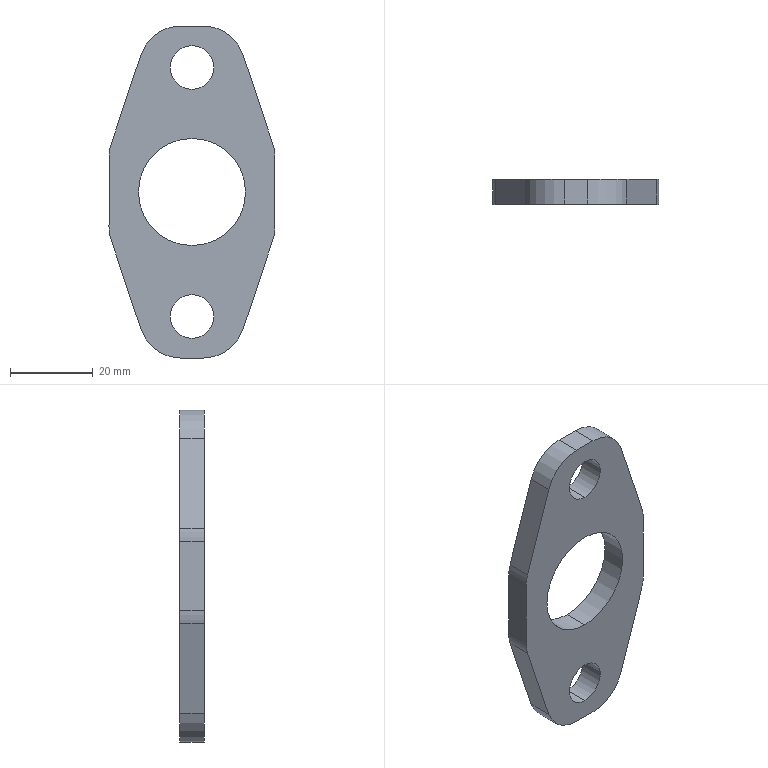Part | SolidWorks | features BaseBody 1 | 1 solid | 24 faces | box 40 x 6 x 80 mm | volume 11190 mm3 | cylinder 14 | plane 10 | commonest cylinder face diameters 20 x8 10.5 x4 25.8 x2
STEP:
#1=CARTESIAN_POINT('',(921.946,-3040.973,882.071));
#2=VERTEX_POINT('',#1);
#3=CARTESIAN_POINT('',(921.946,-3040.973,907.871));
#4=VERTEX_POINT('',#3);
#5=CARTESIAN_POINT('',(921.946,-3040.973,894.971));
#6=DIRECTION('',(0.,1.,0.));
#7=DIRECTION('',(0.,0.,-1.));
#8=AXIS2_PLACEMENT_3D('',#5,#6,#7);
#9=CIRCLE('',#8,12.9);
#10=EDGE_CURVE('',#2,#4,#9,.T.);
#11=ORIENTED_EDGE('',*,*,#10,.T.);
#12=CARTESIAN_POINT('',(921.946,-3046.973,907.871));
#13=VERTEX_POINT('',#12);
#14=CARTESIAN_POINT('',(921.946,-3040.973,907.871));
#15=DIRECTION('',(0.,-1.,0.));
#16=VECTOR('',#15,1000.);
#17=LINE('',#14,#16);
#18=EDGE_CURVE('',#4,#13,#17,.T.);
#19=ORIENTED_EDGE('',*,*,#18,.T.);
#20=CARTESIAN_POINT('',(921.946,-3046.973,882.071));
#21=VERTEX_POINT('',#20);
#22=CARTESIAN_POINT('',(921.946,-3046.973,894.971));
#23=DIRECTION('',(0.,-1.,0.));
#24=DIRECTION('',(0.,0.,-1.));
#25=AXIS2_PLACEMENT_3D('',#22,#23,#24);
#26=CIRCLE('',#25,12.9);
#27=EDGE_CURVE('',#13,#21,#26,.T.);
#28=ORIENTED_EDGE('',*,*,#27,.T.);
#29=CARTESIAN_POINT('',(921.946,-3040.973,882.071));
#30=DIRECTION('',(0.,-1.,0.));
#31=VECTOR('',#30,1000.);
#32=LINE('',#29,#31);
#33=EDGE_CURVE('',#2,#21,#32,.T.);
#34=ORIENTED_EDGE('',*,*,#33,.F.);
#35=EDGE_LOOP('',(#11,#19,#28,#34));
#36=FACE_OUTER_BOUND('',#35,.T.);
#37=CARTESIAN_POINT('',(921.946,-3040.973,894.971));
#38=DIRECTION('',(0.,-1.,0.));
#39=DIRECTION('',(0.,0.,-1.));
#40=AXIS2_PLACEMENT_3D('',#37,#38,#39);
#41=CYLINDRICAL_SURFACE('',#40,12.9);
#42=ADVANCED_FACE('',(#36),#41,.F.);
#43=CARTESIAN_POINT('',(921.946,-3040.973,859.721));
#44=VERTEX_POINT('',#43);
#45=CARTESIAN_POINT('',(921.946,-3040.973,870.221));
#46=VERTEX_POINT('',#45);
#47=CARTESIAN_POINT('',(921.946,-3040.973,864.971));
#48=DIRECTION('',(0.,1.,0.));
#49=DIRECTION('',(0.,0.,-1.));
#50=AXIS2_PLACEMENT_3D('',#47,#48,#49);
#51=CIRCLE('',#50,5.25);
#52=EDGE_CURVE('',#44,#46,#51,.T.);
#53=ORIENTED_EDGE('',*,*,#52,.T.);
#54=CARTESIAN_POINT('',(921.946,-3046.973,870.221));
#55=VERTEX_POINT('',#54);
#56=CARTESIAN_POINT('',(921.946,-3040.973,870.221));
#57=DIRECTION('',(0.,-1.,0.));
#58=VECTOR('',#57,1000.);
#59=LINE('',#56,#58);
#60=EDGE_CURVE('',#46,#55,#59,.T.);
#61=ORIENTED_EDGE('',*,*,#60,.T.);
#62=CARTESIAN_POINT('',(921.946,-3046.973,859.721));
#63=VERTEX_POINT('',#62);
#64=CARTESIAN_POINT('',(921.946,-3046.973,864.971));
#65=DIRECTION('',(0.,-1.,0.));
#66=DIRECTION('',(0.,0.,-1.));
#67=AXIS2_PLACEMENT_3D('',#64,#65,#66);
#68=CIRCLE('',#67,5.25);
#69=EDGE_CURVE('',#55,#63,#68,.T.);
#70=ORIENTED_EDGE('',*,*,#69,.T.);
#71=CARTESIAN_POINT('',(921.946,-3040.973,859.721));
#72=DIRECTION('',(0.,-1.,0.));
#73=VECTOR('',#72,1000.);
#74=LINE('',#71,#73);
#75=EDGE_CURVE('',#44,#63,#74,.T.);
#76=ORIENTED_EDGE('',*,*,#75,.F.);
#77=EDGE_LOOP('',(#53,#61,#70,#76));
#78=FACE_OUTER_BOUND('',#77,.T.);
#79=CARTESIAN_POINT('',(921.946,-3040.973,864.971));
#80=DIRECTION('',(0.,-1.,0.));
#81=DIRECTION('',(0.,0.,-1.));
#82=AXIS2_PLACEMENT_3D('',#79,#80,#81);
#83=CYLINDRICAL_SURFACE('',#82,5.25);
#84=ADVANCED_FACE('',(#78),#83,.F.);
#85=CARTESIAN_POINT('',(921.946,-3040.973,919.721));
#86=VERTEX_POINT('',#85);
#87=CARTESIAN_POINT('',(921.946,-3040.973,930.221));
#88=VERTEX_POINT('',#87);
#89=CARTESIAN_POINT('',(921.946,-3040.973,924.971));
#90=DIRECTION('',(0.,1.,0.));
#91=DIRECTION('',(0.,0.,-1.));
#92=AXIS2_PLACEMENT_3D('',#89,#90,#91);
#93=CIRCLE('',#92,5.25);
#94=EDGE_CURVE('',#86,#88,#93,.T.);
#95=ORIENTED_EDGE('',*,*,#94,.T.);
#96=CARTESIAN_POINT('',(921.946,-3046.973,930.221));
#97=VERTEX_POINT('',#96);
#98=CARTESIAN_POINT('',(921.946,-3040.973,930.221));
#99=DIRECTION('',(0.,-1.,0.));
#100=VECTOR('',#99,1000.);
#101=LINE('',#98,#100);
#102=EDGE_CURVE('',#88,#97,#101,.T.);
#103=ORIENTED_EDGE('',*,*,#102,.T.);
#104=CARTESIAN_POINT('',(921.946,-3046.973,919.721));
#105=VERTEX_POINT('',#104);
#106=CARTESIAN_POINT('',(921.946,-3046.973,924.971));
#107=DIRECTION('',(0.,-1.,0.));
#108=DIRECTION('',(0.,0.,-1.));
#109=AXIS2_PLACEMENT_3D('',#106,#107,#108);
#110=CIRCLE('',#109,5.25);
#111=EDGE_CURVE('',#97,#105,#110,.T.);
#112=ORIENTED_EDGE('',*,*,#111,.T.);
#113=CARTESIAN_POINT('',(921.946,-3040.973,919.721));
#114=DIRECTION('',(0.,-1.,0.));
#115=VECTOR('',#114,1000.);
#116=LINE('',#113,#115);
#117=EDGE_CURVE('',#86,#105,#116,.T.);
#118=ORIENTED_EDGE('',*,*,#117,.F.);
#119=EDGE_LOOP('',(#95,#103,#112,#118));
#120=FACE_OUTER_BOUND('',#119,.T.);
#121=CARTESIAN_POINT('',(921.946,-3040.973,924.971));
#122=DIRECTION('',(0.,-1.,0.));
#123=DIRECTION('',(0.,0.,-1.));
#124=AXIS2_PLACEMENT_3D('',#121,#122,#123);
#125=CYLINDRICAL_SURFACE('',#124,5.25);
#126=ADVANCED_FACE('',(#120),#125,.F.);
#127=CARTESIAN_POINT('',(941.946,-3046.973,886.594));
#128=VERTEX_POINT('',#127);
#129=CARTESIAN_POINT('',(941.432,-3046.973,883.432));
#130=VERTEX_POINT('',#129);
#131=CARTESIAN_POINT('',(931.946,-3046.973,886.594));
#132=DIRECTION('',(0.,1.,0.));
#133=DIRECTION('',(0.,0.,-1.));
#134=AXIS2_PLACEMENT_3D('',#131,#132,#133);
#135=CIRCLE('',#134,10.);
#136=EDGE_CURVE('',#128,#130,#135,.T.);
#137=ORIENTED_EDGE('',*,*,#136,.F.);
#138=CARTESIAN_POINT('',(941.946,-3046.973,903.349));
#139=VERTEX_POINT('',#138);
#140=CARTESIAN_POINT('',(941.946,-3046.973,894.971));
#141=DIRECTION('',(0.,0.,-1.));
#142=VECTOR('',#141,1000.);
#143=LINE('',#140,#142);
#144=EDGE_CURVE('',#139,#128,#143,.T.);
#145=ORIENTED_EDGE('',*,*,#144,.F.);
#146=CARTESIAN_POINT('',(941.432,-3046.973,906.511));
#147=VERTEX_POINT('',#146);
#148=CARTESIAN_POINT('',(931.946,-3046.973,903.349));
#149=DIRECTION('',(0.,1.,0.));
#150=DIRECTION('',(0.,0.,-1.));
#151=AXIS2_PLACEMENT_3D('',#148,#149,#150);
#152=CIRCLE('',#151,10.);
#153=EDGE_CURVE('',#147,#139,#152,.T.);
#154=ORIENTED_EDGE('',*,*,#153,.F.);
#155=CARTESIAN_POINT('',(934.225,-3046.973,928.134));
#156=VERTEX_POINT('',#155);
#157=CARTESIAN_POINT('',(934.225,-3046.973,928.134));
#158=DIRECTION('',(0.3162,0.,-0.9487));
#159=VECTOR('',#158,1000.);
#160=LINE('',#157,#159);
#161=EDGE_CURVE('',#156,#147,#160,.T.);
#162=ORIENTED_EDGE('',*,*,#161,.F.);
#163=CARTESIAN_POINT('',(924.738,-3046.973,934.971));
#164=VERTEX_POINT('',#163);
#165=CARTESIAN_POINT('',(924.738,-3046.973,924.971));
#166=DIRECTION('',(0.,1.,0.));
#167=DIRECTION('',(0.,0.,-1.));
#168=AXIS2_PLACEMENT_3D('',#165,#166,#167);
#169=CIRCLE('',#168,10.);
#170=EDGE_CURVE('',#164,#156,#169,.T.);
#171=ORIENTED_EDGE('',*,*,#170,.F.);
#172=CARTESIAN_POINT('',(919.153,-3046.973,934.971));
#173=VERTEX_POINT('',#172);
#174=CARTESIAN_POINT('',(921.946,-3046.973,934.971));
#175=DIRECTION('',(1.,0.,0.));
#176=VECTOR('',#175,1000.);
#177=LINE('',#174,#176);
#178=EDGE_CURVE('',#173,#164,#177,.T.);
#179=ORIENTED_EDGE('',*,*,#178,.F.);
#180=CARTESIAN_POINT('',(909.666,-3046.973,928.134));
#181=VERTEX_POINT('',#180);
#182=CARTESIAN_POINT('',(919.153,-3046.973,924.971));
#183=DIRECTION('',(0.,1.,0.));
#184=DIRECTION('',(0.,0.,-1.));
#185=AXIS2_PLACEMENT_3D('',#182,#183,#184);
#186=CIRCLE('',#185,10.);
#187=EDGE_CURVE('',#181,#173,#186,.T.);
#188=ORIENTED_EDGE('',*,*,#187,.F.);
#189=CARTESIAN_POINT('',(902.459,-3046.973,906.511));
#190=VERTEX_POINT('',#189);
#191=CARTESIAN_POINT('',(902.459,-3046.973,906.511));
#192=DIRECTION('',(0.3162,0.,0.9487));
#193=VECTOR('',#192,1000.);
#194=LINE('',#191,#193);
#195=EDGE_CURVE('',#190,#181,#194,.T.);
#196=ORIENTED_EDGE('',*,*,#195,.F.);
#197=CARTESIAN_POINT('',(901.946,-3046.973,903.349));
#198=VERTEX_POINT('',#197);
#199=CARTESIAN_POINT('',(911.946,-3046.973,903.349));
#200=DIRECTION('',(0.,1.,0.));
#201=DIRECTION('',(0.,0.,-1.));
#202=AXIS2_PLACEMENT_3D('',#199,#200,#201);
#203=CIRCLE('',#202,10.);
#204=EDGE_CURVE('',#198,#190,#203,.T.);
#205=ORIENTED_EDGE('',*,*,#204,.F.);
#206=CARTESIAN_POINT('',(901.946,-3046.973,886.594));
#207=VERTEX_POINT('',#206);
#208=CARTESIAN_POINT('',(901.946,-3046.973,894.971));
#209=DIRECTION('',(0.,0.,1.));
#210=VECTOR('',#209,1000.);
#211=LINE('',#208,#210);
#212=EDGE_CURVE('',#207,#198,#211,.T.);
#213=ORIENTED_EDGE('',*,*,#212,.F.);
#214=CARTESIAN_POINT('',(902.459,-3046.973,883.432));
#215=VERTEX_POINT('',#214);
#216=CARTESIAN_POINT('',(911.946,-3046.973,886.594));
#217=DIRECTION('',(0.,1.,0.));
#218=DIRECTION('',(0.,0.,-1.));
#219=AXIS2_PLACEMENT_3D('',#216,#217,#218);
#220=CIRCLE('',#219,10.);
#221=EDGE_CURVE('',#215,#207,#220,.T.);
#222=ORIENTED_EDGE('',*,*,#221,.F.);
#223=CARTESIAN_POINT('',(909.666,-3046.973,861.809));
#224=VERTEX_POINT('',#223);
#225=CARTESIAN_POINT('',(909.666,-3046.973,861.809));
#226=DIRECTION('',(-0.3162,0.,0.9487));
#227=VECTOR('',#226,1000.);
#228=LINE('',#225,#227);
#229=EDGE_CURVE('',#224,#215,#228,.T.);
#230=ORIENTED_EDGE('',*,*,#229,.F.);
#231=CARTESIAN_POINT('',(919.153,-3046.973,854.971));
#232=VERTEX_POINT('',#231);
#233=CARTESIAN_POINT('',(919.153,-3046.973,864.971));
#234=DIRECTION('',(0.,1.,0.));
#235=DIRECTION('',(0.,0.,-1.));
#236=AXIS2_PLACEMENT_3D('',#233,#234,#235);
#237=CIRCLE('',#236,10.);
#238=EDGE_CURVE('',#232,#224,#237,.T.);
#239=ORIENTED_EDGE('',*,*,#238,.F.);
#240=CARTESIAN_POINT('',(924.738,-3046.973,854.971));
#241=VERTEX_POINT('',#240);
#242=CARTESIAN_POINT('',(921.946,-3046.973,854.971));
#243=DIRECTION('',(-1.,0.,0.));
#244=VECTOR('',#243,1000.);
#245=LINE('',#242,#244);
#246=EDGE_CURVE('',#241,#232,#245,.T.);
#247=ORIENTED_EDGE('',*,*,#246,.F.);
#248=CARTESIAN_POINT('',(934.225,-3046.973,861.809));
#249=VERTEX_POINT('',#248);
#250=CARTESIAN_POINT('',(924.738,-3046.973,864.971));
#251=DIRECTION('',(0.,1.,0.));
#252=DIRECTION('',(0.,0.,-1.));
#253=AXIS2_PLACEMENT_3D('',#250,#251,#252);
#254=CIRCLE('',#253,10.);
#255=EDGE_CURVE('',#249,#241,#254,.T.);
#256=ORIENTED_EDGE('',*,*,#255,.F.);
#257=CARTESIAN_POINT('',(941.432,-3046.973,883.432));
#258=DIRECTION('',(-0.3162,0.,-0.9487));
#259=VECTOR('',#258,1000.);
#260=LINE('',#257,#259);
#261=EDGE_CURVE('',#130,#249,#260,.T.);
#262=ORIENTED_EDGE('',*,*,#261,.F.);
#263=EDGE_LOOP('',(#137,#145,#154,#162,#171,#179,#188,#196,#205,#213,#222,#230,#239,#247,#256,#262));
#264=FACE_OUTER_BOUND('',#263,.T.);
#265=CARTESIAN_POINT('',(921.946,-3046.973,894.971));
#266=DIRECTION('',(0.,-1.,0.));
#267=DIRECTION('',(0.,0.,-1.));
#268=AXIS2_PLACEMENT_3D('',#265,#266,#267);
#269=CIRCLE('',#268,12.9);
#270=EDGE_CURVE('',#21,#13,#269,.T.);
#271=ORIENTED_EDGE('',*,*,#270,.F.);
#272=ORIENTED_EDGE('',*,*,#27,.F.);
#273=EDGE_LOOP('',(#271,#272));
#274=FACE_BOUND('',#273,.T.);
#275=CARTESIAN_POINT('',(921.946,-3046.973,864.971));
#276=DIRECTION('',(0.,-1.,0.));
#277=DIRECTION('',(0.,0.,-1.));
#278=AXIS2_PLACEMENT_3D('',#275,#276,#277);
#279=CIRCLE('',#278,5.25);
#280=EDGE_CURVE('',#63,#55,#279,.T.);
#281=ORIENTED_EDGE('',*,*,#280,.F.);
#282=ORIENTED_EDGE('',*,*,#69,.F.);
#283=EDGE_LOOP('',(#281,#282));
#284=FACE_BOUND('',#283,.T.);
#285=CARTESIAN_POINT('',(921.946,-3046.973,924.971));
#286=DIRECTION('',(0.,-1.,0.));
#287=DIRECTION('',(0.,0.,-1.));
#288=AXIS2_PLACEMENT_3D('',#285,#286,#287);
#289=CIRCLE('',#288,5.25);
#290=EDGE_CURVE('',#105,#97,#289,.T.);
#291=ORIENTED_EDGE('',*,*,#290,.F.);
#292=ORIENTED_EDGE('',*,*,#111,.F.);
#293=EDGE_LOOP('',(#291,#292));
#294=FACE_BOUND('',#293,.T.);
#295=CARTESIAN_POINT('',(921.946,-3046.973,894.971));
#296=DIRECTION('',(0.,1.,0.));
#297=DIRECTION('',(0.,0.,1.));
#298=AXIS2_PLACEMENT_3D('',#295,#296,#297);
#299=PLANE('',#298);
#300=ADVANCED_FACE('',(#264,#274,#284,#294),#299,.F.);
#301=CARTESIAN_POINT('',(934.225,-3040.973,861.809));
#302=VERTEX_POINT('',#301);
#303=CARTESIAN_POINT('',(941.432,-3040.973,883.432));
#304=VERTEX_POINT('',#303);
#305=CARTESIAN_POINT('',(941.432,-3040.973,883.432));
#306=DIRECTION('',(0.3162,0.,0.9487));
#307=VECTOR('',#306,1000.);
#308=LINE('',#305,#307);
#309=EDGE_CURVE('',#302,#304,#308,.T.);
#310=ORIENTED_EDGE('',*,*,#309,.T.);
#311=CARTESIAN_POINT('',(941.432,-3040.973,883.432));
#312=DIRECTION('',(0.,-1.,0.));
#313=VECTOR('',#312,1000.);
#314=LINE('',#311,#313);
#315=EDGE_CURVE('',#304,#130,#314,.T.);
#316=ORIENTED_EDGE('',*,*,#315,.T.);
#317=ORIENTED_EDGE('',*,*,#261,.T.);
#318=CARTESIAN_POINT('',(934.225,-3040.973,861.809));
#319=DIRECTION('',(0.,1.,0.));
#320=VECTOR('',#319,1000.);
#321=LINE('',#318,#320);
#322=EDGE_CURVE('',#249,#302,#321,.T.);
#323=ORIENTED_EDGE('',*,*,#322,.T.);
#324=EDGE_LOOP('',(#310,#316,#317,#323));
#325=FACE_OUTER_BOUND('',#324,.T.);
#326=CARTESIAN_POINT('',(941.432,-3040.973,883.432));
#327=DIRECTION('',(0.9487,0.,-0.3162));
#328=DIRECTION('',(-0.3162,0.,-0.9487));
#329=AXIS2_PLACEMENT_3D('',#326,#327,#328);
#330=PLANE('',#329);
#331=ADVANCED_FACE('',(#325),#330,.T.);
#332=CARTESIAN_POINT('',(941.946,-3040.973,886.594));
#333=VERTEX_POINT('',#332);
#334=CARTESIAN_POINT('',(931.946,-3040.973,886.594));
#335=DIRECTION('',(0.,-1.,0.));
#336=DIRECTION('',(0.,0.,-1.));
#337=AXIS2_PLACEMENT_3D('',#334,#335,#336);
#338=CIRCLE('',#337,10.);
#339=EDGE_CURVE('',#304,#333,#338,.T.);
#340=ORIENTED_EDGE('',*,*,#339,.T.);
#341=CARTESIAN_POINT('',(941.946,-3040.973,886.594));
#342=DIRECTION('',(0.,-1.,0.));
#343=VECTOR('',#342,1000.);
#344=LINE('',#341,#343);
#345=EDGE_CURVE('',#333,#128,#344,.T.);
#346=ORIENTED_EDGE('',*,*,#345,.T.);
#347=ORIENTED_EDGE('',*,*,#136,.T.);
#348=ORIENTED_EDGE('',*,*,#315,.F.);
#349=EDGE_LOOP('',(#340,#346,#347,#348));
#350=FACE_OUTER_BOUND('',#349,.T.);
#351=CARTESIAN_POINT('',(931.946,-3040.973,886.594));
#352=DIRECTION('',(0.,-1.,0.));
#353=DIRECTION('',(0.,0.,-1.));
#354=AXIS2_PLACEMENT_3D('',#351,#352,#353);
#355=CYLINDRICAL_SURFACE('',#354,10.);
#356=ADVANCED_FACE('',(#350),#355,.T.);
#357=CARTESIAN_POINT('',(941.946,-3040.973,903.349));
#358=VERTEX_POINT('',#357);
#359=CARTESIAN_POINT('',(941.946,-3040.973,903.349));
#360=DIRECTION('',(0.,0.,1.));
#361=VECTOR('',#360,1000.);
#362=LINE('',#359,#361);
#363=EDGE_CURVE('',#333,#358,#362,.T.);
#364=ORIENTED_EDGE('',*,*,#363,.T.);
#365=CARTESIAN_POINT('',(941.946,-3040.973,903.349));
#366=DIRECTION('',(0.,-1.,0.));
#367=VECTOR('',#366,1000.);
#368=LINE('',#365,#367);
#369=EDGE_CURVE('',#358,#139,#368,.T.);
#370=ORIENTED_EDGE('',*,*,#369,.T.);
#371=ORIENTED_EDGE('',*,*,#144,.T.);
#372=ORIENTED_EDGE('',*,*,#345,.F.);
#373=EDGE_LOOP('',(#364,#370,#371,#372));
#374=FACE_OUTER_BOUND('',#373,.T.);
#375=CARTESIAN_POINT('',(941.946,-3040.973,903.349));
#376=DIRECTION('',(1.,0.,0.));
#377=DIRECTION('',(0.,1.,0.));
#378=AXIS2_PLACEMENT_3D('',#375,#376,#377);
#379=PLANE('',#378);
#380=ADVANCED_FACE('',(#374),#379,.T.);
#381=CARTESIAN_POINT('',(941.432,-3040.973,906.511));
#382=VERTEX_POINT('',#381);
#383=CARTESIAN_POINT('',(931.946,-3040.973,903.349));
#384=DIRECTION('',(0.,-1.,0.));
#385=DIRECTION('',(0.,0.,-1.));
#386=AXIS2_PLACEMENT_3D('',#383,#384,#385);
#387=CIRCLE('',#386,10.);
#388=EDGE_CURVE('',#358,#382,#387,.T.);
#389=ORIENTED_EDGE('',*,*,#388,.T.);
#390=CARTESIAN_POINT('',(941.432,-3040.973,906.511));
#391=DIRECTION('',(0.,-1.,0.));
#392=VECTOR('',#391,1000.);
#393=LINE('',#390,#392);
#394=EDGE_CURVE('',#382,#147,#393,.T.);
#395=ORIENTED_EDGE('',*,*,#394,.T.);
#396=ORIENTED_EDGE('',*,*,#153,.T.);
#397=ORIENTED_EDGE('',*,*,#369,.F.);
#398=EDGE_LOOP('',(#389,#395,#396,#397));
#399=FACE_OUTER_BOUND('',#398,.T.);
#400=CARTESIAN_POINT('',(931.946,-3040.973,903.349));
#401=DIRECTION('',(0.,-1.,0.));
#402=DIRECTION('',(0.,0.,-1.));
#403=AXIS2_PLACEMENT_3D('',#400,#401,#402);
#404=CYLINDRICAL_SURFACE('',#403,10.);
#405=ADVANCED_FACE('',(#399),#404,.T.);
#406=CARTESIAN_POINT('',(934.225,-3040.973,928.134));
#407=VERTEX_POINT('',#406);
#408=CARTESIAN_POINT('',(934.225,-3040.973,928.134));
#409=DIRECTION('',(-0.3162,0.,0.9487));
#410=VECTOR('',#409,1000.);
#411=LINE('',#408,#410);
#412=EDGE_CURVE('',#382,#407,#411,.T.);
#413=ORIENTED_EDGE('',*,*,#412,.T.);
#414=CARTESIAN_POINT('',(934.225,-3040.973,928.134));
#415=DIRECTION('',(0.,-1.,0.));
#416=VECTOR('',#415,1000.);
#417=LINE('',#414,#416);
#418=EDGE_CURVE('',#407,#156,#417,.T.);
#419=ORIENTED_EDGE('',*,*,#418,.T.);
#420=ORIENTED_EDGE('',*,*,#161,.T.);
#421=ORIENTED_EDGE('',*,*,#394,.F.);
#422=EDGE_LOOP('',(#413,#419,#420,#421));
#423=FACE_OUTER_BOUND('',#422,.T.);
#424=CARTESIAN_POINT('',(934.225,-3040.973,928.134));
#425=DIRECTION('',(0.9487,0.,0.3162));
#426=DIRECTION('',(0.3162,0.,-0.9487));
#427=AXIS2_PLACEMENT_3D('',#424,#425,#426);
#428=PLANE('',#427);
#429=ADVANCED_FACE('',(#423),#428,.T.);
#430=CARTESIAN_POINT('',(924.738,-3040.973,934.971));
#431=VERTEX_POINT('',#430);
#432=CARTESIAN_POINT('',(924.738,-3040.973,924.971));
#433=DIRECTION('',(0.,-1.,0.));
#434=DIRECTION('',(0.,0.,-1.));
#435=AXIS2_PLACEMENT_3D('',#432,#433,#434);
#436=CIRCLE('',#435,10.);
#437=EDGE_CURVE('',#407,#431,#436,.T.);
#438=ORIENTED_EDGE('',*,*,#437,.T.);
#439=CARTESIAN_POINT('',(924.738,-3040.973,934.971));
#440=DIRECTION('',(0.,-1.,0.));
#441=VECTOR('',#440,1000.);
#442=LINE('',#439,#441);
#443=EDGE_CURVE('',#431,#164,#442,.T.);
#444=ORIENTED_EDGE('',*,*,#443,.T.);
#445=ORIENTED_EDGE('',*,*,#170,.T.);
#446=ORIENTED_EDGE('',*,*,#418,.F.);
#447=EDGE_LOOP('',(#438,#444,#445,#446));
#448=FACE_OUTER_BOUND('',#447,.T.);
#449=CARTESIAN_POINT('',(924.738,-3040.973,924.971));
#450=DIRECTION('',(0.,-1.,0.));
#451=DIRECTION('',(0.,0.,-1.));
#452=AXIS2_PLACEMENT_3D('',#449,#450,#451);
#453=CYLINDRICAL_SURFACE('',#452,10.);
#454=ADVANCED_FACE('',(#448),#453,.T.);
#455=CARTESIAN_POINT('',(919.153,-3040.973,934.971));
#456=VERTEX_POINT('',#455);
#457=CARTESIAN_POINT('',(919.153,-3040.973,934.971));
#458=DIRECTION('',(-1.,0.,0.));
#459=VECTOR('',#458,1000.);
#460=LINE('',#457,#459);
#461=EDGE_CURVE('',#431,#456,#460,.T.);
#462=ORIENTED_EDGE('',*,*,#461,.T.);
#463=CARTESIAN_POINT('',(919.153,-3040.973,934.971));
#464=DIRECTION('',(0.,-1.,0.));
#465=VECTOR('',#464,1000.);
#466=LINE('',#463,#465);
#467=EDGE_CURVE('',#456,#173,#466,.T.);
#468=ORIENTED_EDGE('',*,*,#467,.T.);
#469=ORIENTED_EDGE('',*,*,#178,.T.);
#470=ORIENTED_EDGE('',*,*,#443,.F.);
#471=EDGE_LOOP('',(#462,#468,#469,#470));
#472=FACE_OUTER_BOUND('',#471,.T.);
#473=CARTESIAN_POINT('',(919.153,-3040.973,934.971));
#474=DIRECTION('',(0.,0.,1.));
#475=DIRECTION('',(0.,-1.,0.));
#476=AXIS2_PLACEMENT_3D('',#473,#474,#475);
#477=PLANE('',#476);
#478=ADVANCED_FACE('',(#472),#477,.T.);
#479=CARTESIAN_POINT('',(909.666,-3040.973,928.134));
#480=VERTEX_POINT('',#479);
#481=CARTESIAN_POINT('',(919.153,-3040.973,924.971));
#482=DIRECTION('',(0.,-1.,0.));
#483=DIRECTION('',(0.,0.,-1.));
#484=AXIS2_PLACEMENT_3D('',#481,#482,#483);
#485=CIRCLE('',#484,10.);
#486=EDGE_CURVE('',#456,#480,#485,.T.);
#487=ORIENTED_EDGE('',*,*,#486,.T.);
#488=CARTESIAN_POINT('',(909.666,-3040.973,928.134));
#489=DIRECTION('',(0.,-1.,0.));
#490=VECTOR('',#489,1000.);
#491=LINE('',#488,#490);
#492=EDGE_CURVE('',#480,#181,#491,.T.);
#493=ORIENTED_EDGE('',*,*,#492,.T.);
#494=ORIENTED_EDGE('',*,*,#187,.T.);
#495=ORIENTED_EDGE('',*,*,#467,.F.);
#496=EDGE_LOOP('',(#487,#493,#494,#495));
#497=FACE_OUTER_BOUND('',#496,.T.);
#498=CARTESIAN_POINT('',(919.153,-3040.973,924.971));
#499=DIRECTION('',(0.,-1.,0.));
#500=DIRECTION('',(0.,0.,-1.));
#501=AXIS2_PLACEMENT_3D('',#498,#499,#500);
#502=CYLINDRICAL_SURFACE('',#501,10.);
#503=ADVANCED_FACE('',(#497),#502,.T.);
#504=CARTESIAN_POINT('',(902.459,-3040.973,906.511));
#505=VERTEX_POINT('',#504);
#506=CARTESIAN_POINT('',(902.459,-3040.973,906.511));
#507=DIRECTION('',(-0.3162,0.,-0.9487));
#508=VECTOR('',#507,1000.);
#509=LINE('',#506,#508);
#510=EDGE_CURVE('',#480,#505,#509,.T.);
#511=ORIENTED_EDGE('',*,*,#510,.T.);
#512=CARTESIAN_POINT('',(902.459,-3040.973,906.511));
#513=DIRECTION('',(0.,-1.,0.));
#514=VECTOR('',#513,1000.);
#515=LINE('',#512,#514);
#516=EDGE_CURVE('',#505,#190,#515,.T.);
#517=ORIENTED_EDGE('',*,*,#516,.T.);
#518=ORIENTED_EDGE('',*,*,#195,.T.);
#519=ORIENTED_EDGE('',*,*,#492,.F.);
#520=EDGE_LOOP('',(#511,#517,#518,#519));
#521=FACE_OUTER_BOUND('',#520,.T.);
#522=CARTESIAN_POINT('',(902.459,-3040.973,906.511));
#523=DIRECTION('',(-0.9487,0.,0.3162));
#524=DIRECTION('',(0.3162,0.,0.9487));
#525=AXIS2_PLACEMENT_3D('',#522,#523,#524);
#526=PLANE('',#525);
#527=ADVANCED_FACE('',(#521),#526,.T.);
#528=CARTESIAN_POINT('',(901.946,-3040.973,903.349));
#529=VERTEX_POINT('',#528);
#530=CARTESIAN_POINT('',(911.946,-3040.973,903.349));
#531=DIRECTION('',(0.,-1.,0.));
#532=DIRECTION('',(0.,0.,-1.));
#533=AXIS2_PLACEMENT_3D('',#530,#531,#532);
#534=CIRCLE('',#533,10.);
#535=EDGE_CURVE('',#505,#529,#534,.T.);
#536=ORIENTED_EDGE('',*,*,#535,.T.);
#537=CARTESIAN_POINT('',(901.946,-3040.973,903.349));
#538=DIRECTION('',(0.,-1.,0.));
#539=VECTOR('',#538,1000.);
#540=LINE('',#537,#539);
#541=EDGE_CURVE('',#529,#198,#540,.T.);
#542=ORIENTED_EDGE('',*,*,#541,.T.);
#543=ORIENTED_EDGE('',*,*,#204,.T.);
#544=ORIENTED_EDGE('',*,*,#516,.F.);
#545=EDGE_LOOP('',(#536,#542,#543,#544));
#546=FACE_OUTER_BOUND('',#545,.T.);
#547=CARTESIAN_POINT('',(911.946,-3040.973,903.349));
#548=DIRECTION('',(0.,-1.,0.));
#549=DIRECTION('',(0.,0.,-1.));
#550=AXIS2_PLACEMENT_3D('',#547,#548,#549);
#551=CYLINDRICAL_SURFACE('',#550,10.);
#552=ADVANCED_FACE('',(#546),#551,.T.);
#553=CARTESIAN_POINT('',(901.946,-3040.973,886.594));
#554=VERTEX_POINT('',#553);
#555=CARTESIAN_POINT('',(901.946,-3040.973,886.594));
#556=DIRECTION('',(0.,0.,-1.));
#557=VECTOR('',#556,1000.);
#558=LINE('',#555,#557);
#559=EDGE_CURVE('',#529,#554,#558,.T.);
#560=ORIENTED_EDGE('',*,*,#559,.T.);
#561=CARTESIAN_POINT('',(901.946,-3040.973,886.594));
#562=DIRECTION('',(0.,-1.,0.));
#563=VECTOR('',#562,1000.);
#564=LINE('',#561,#563);
#565=EDGE_CURVE('',#554,#207,#564,.T.);
#566=ORIENTED_EDGE('',*,*,#565,.T.);
#567=ORIENTED_EDGE('',*,*,#212,.T.);
#568=ORIENTED_EDGE('',*,*,#541,.F.);
#569=EDGE_LOOP('',(#560,#566,#567,#568));
#570=FACE_OUTER_BOUND('',#569,.T.);
#571=CARTESIAN_POINT('',(901.946,-3040.973,886.594));
#572=DIRECTION('',(-1.,0.,0.));
#573=DIRECTION('',(0.,0.,1.));
#574=AXIS2_PLACEMENT_3D('',#571,#572,#573);
#575=PLANE('',#574);
#576=ADVANCED_FACE('',(#570),#575,.T.);
#577=CARTESIAN_POINT('',(902.459,-3040.973,883.432));
#578=VERTEX_POINT('',#577);
#579=CARTESIAN_POINT('',(911.946,-3040.973,886.594));
#580=DIRECTION('',(0.,-1.,0.));
#581=DIRECTION('',(0.,0.,-1.));
#582=AXIS2_PLACEMENT_3D('',#579,#580,#581);
#583=CIRCLE('',#582,10.);
#584=EDGE_CURVE('',#554,#578,#583,.T.);
#585=ORIENTED_EDGE('',*,*,#584,.T.);
#586=CARTESIAN_POINT('',(902.459,-3040.973,883.432));
#587=DIRECTION('',(0.,-1.,0.));
#588=VECTOR('',#587,1000.);
#589=LINE('',#586,#588);
#590=EDGE_CURVE('',#578,#215,#589,.T.);
#591=ORIENTED_EDGE('',*,*,#590,.T.);
#592=ORIENTED_EDGE('',*,*,#221,.T.);
#593=ORIENTED_EDGE('',*,*,#565,.F.);
#594=EDGE_LOOP('',(#585,#591,#592,#593));
#595=FACE_OUTER_BOUND('',#594,.T.);
#596=CARTESIAN_POINT('',(911.946,-3040.973,886.594));
#597=DIRECTION('',(0.,-1.,0.));
#598=DIRECTION('',(0.,0.,-1.));
#599=AXIS2_PLACEMENT_3D('',#596,#597,#598);
#600=CYLINDRICAL_SURFACE('',#599,10.);
#601=ADVANCED_FACE('',(#595),#600,.T.);
#602=CARTESIAN_POINT('',(909.666,-3040.973,861.809));
#603=VERTEX_POINT('',#602);
#604=CARTESIAN_POINT('',(909.666,-3040.973,861.809));
#605=DIRECTION('',(0.3162,0.,-0.9487));
#606=VECTOR('',#605,1000.);
#607=LINE('',#604,#606);
#608=EDGE_CURVE('',#578,#603,#607,.T.);
#609=ORIENTED_EDGE('',*,*,#608,.T.);
#610=CARTESIAN_POINT('',(909.666,-3040.973,861.809));
#611=DIRECTION('',(0.,-1.,0.));
#612=VECTOR('',#611,1000.);
#613=LINE('',#610,#612);
#614=EDGE_CURVE('',#603,#224,#613,.T.);
#615=ORIENTED_EDGE('',*,*,#614,.T.);
#616=ORIENTED_EDGE('',*,*,#229,.T.);
#617=ORIENTED_EDGE('',*,*,#590,.F.);
#618=EDGE_LOOP('',(#609,#615,#616,#617));
#619=FACE_OUTER_BOUND('',#618,.T.);
#620=CARTESIAN_POINT('',(909.666,-3040.973,861.809));
#621=DIRECTION('',(-0.9487,0.,-0.3162));
#622=DIRECTION('',(-0.3162,0.,0.9487));
#623=AXIS2_PLACEMENT_3D('',#620,#621,#622);
#624=PLANE('',#623);
#625=ADVANCED_FACE('',(#619),#624,.T.);
#626=CARTESIAN_POINT('',(919.153,-3040.973,854.971));
#627=VERTEX_POINT('',#626);
#628=CARTESIAN_POINT('',(919.153,-3040.973,864.971));
#629=DIRECTION('',(0.,-1.,0.));
#630=DIRECTION('',(0.,0.,-1.));
#631=AXIS2_PLACEMENT_3D('',#628,#629,#630);
#632=CIRCLE('',#631,10.);
#633=EDGE_CURVE('',#603,#627,#632,.T.);
#634=ORIENTED_EDGE('',*,*,#633,.T.);
#635=CARTESIAN_POINT('',(919.153,-3040.973,854.971));
#636=DIRECTION('',(0.,-1.,0.));
#637=VECTOR('',#636,1000.);
#638=LINE('',#635,#637);
#639=EDGE_CURVE('',#627,#232,#638,.T.);
#640=ORIENTED_EDGE('',*,*,#639,.T.);
#641=ORIENTED_EDGE('',*,*,#238,.T.);
#642=ORIENTED_EDGE('',*,*,#614,.F.);
#643=EDGE_LOOP('',(#634,#640,#641,#642));
#644=FACE_OUTER_BOUND('',#643,.T.);
#645=CARTESIAN_POINT('',(919.153,-3040.973,864.971));
#646=DIRECTION('',(0.,-1.,0.));
#647=DIRECTION('',(0.,0.,-1.));
#648=AXIS2_PLACEMENT_3D('',#645,#646,#647);
#649=CYLINDRICAL_SURFACE('',#648,10.);
#650=ADVANCED_FACE('',(#644),#649,.T.);
#651=CARTESIAN_POINT('',(924.738,-3040.973,854.971));
#652=VERTEX_POINT('',#651);
#653=CARTESIAN_POINT('',(924.738,-3040.973,854.971));
#654=DIRECTION('',(1.,0.,0.));
#655=VECTOR('',#654,1000.);
#656=LINE('',#653,#655);
#657=EDGE_CURVE('',#627,#652,#656,.T.);
#658=ORIENTED_EDGE('',*,*,#657,.T.);
#659=CARTESIAN_POINT('',(924.738,-3040.973,854.971));
#660=DIRECTION('',(0.,-1.,0.));
#661=VECTOR('',#660,1000.);
#662=LINE('',#659,#661);
#663=EDGE_CURVE('',#652,#241,#662,.T.);
#664=ORIENTED_EDGE('',*,*,#663,.T.);
#665=ORIENTED_EDGE('',*,*,#246,.T.);
#666=ORIENTED_EDGE('',*,*,#639,.F.);
#667=EDGE_LOOP('',(#658,#664,#665,#666));
#668=FACE_OUTER_BOUND('',#667,.T.);
#669=CARTESIAN_POINT('',(924.738,-3040.973,854.971));
#670=DIRECTION('',(0.,0.,-1.));
#671=DIRECTION('',(-1.,0.,0.));
#672=AXIS2_PLACEMENT_3D('',#669,#670,#671);
#673=PLANE('',#672);
#674=ADVANCED_FACE('',(#668),#673,.T.);
#675=CARTESIAN_POINT('',(924.738,-3040.973,864.971));
#676=DIRECTION('',(0.,-1.,0.));
#677=DIRECTION('',(0.,0.,-1.));
#678=AXIS2_PLACEMENT_3D('',#675,#676,#677);
#679=CIRCLE('',#678,10.);
#680=EDGE_CURVE('',#652,#302,#679,.T.);
#681=ORIENTED_EDGE('',*,*,#680,.T.);
#682=ORIENTED_EDGE('',*,*,#322,.F.);
#683=ORIENTED_EDGE('',*,*,#255,.T.);
#684=ORIENTED_EDGE('',*,*,#663,.F.);
#685=EDGE_LOOP('',(#681,#682,#683,#684));
#686=FACE_OUTER_BOUND('',#685,.T.);
#687=CARTESIAN_POINT('',(924.738,-3040.973,864.971));
#688=DIRECTION('',(0.,-1.,0.));
#689=DIRECTION('',(0.,0.,-1.));
#690=AXIS2_PLACEMENT_3D('',#687,#688,#689);
#691=CYLINDRICAL_SURFACE('',#690,10.);
#692=ADVANCED_FACE('',(#686),#691,.T.);
#693=ORIENTED_EDGE('',*,*,#18,.F.);
#694=CARTESIAN_POINT('',(921.946,-3040.973,894.971));
#695=DIRECTION('',(0.,1.,0.));
#696=DIRECTION('',(0.,0.,-1.));
#697=AXIS2_PLACEMENT_3D('',#694,#695,#696);
#698=CIRCLE('',#697,12.9);
#699=EDGE_CURVE('',#4,#2,#698,.T.);
#700=ORIENTED_EDGE('',*,*,#699,.T.);
#701=ORIENTED_EDGE('',*,*,#33,.T.);
#702=ORIENTED_EDGE('',*,*,#270,.T.);
#703=EDGE_LOOP('',(#693,#700,#701,#702));
#704=FACE_OUTER_BOUND('',#703,.T.);
#705=CARTESIAN_POINT('',(921.946,-3040.973,894.971));
#706=DIRECTION('',(0.,-1.,0.));
#707=DIRECTION('',(0.,0.,-1.));
#708=AXIS2_PLACEMENT_3D('',#705,#706,#707);
#709=CYLINDRICAL_SURFACE('',#708,12.9);
#710=ADVANCED_FACE('',(#704),#709,.F.);
#711=ORIENTED_EDGE('',*,*,#60,.F.);
#712=CARTESIAN_POINT('',(921.946,-3040.973,864.971));
#713=DIRECTION('',(0.,1.,0.));
#714=DIRECTION('',(0.,0.,-1.));
#715=AXIS2_PLACEMENT_3D('',#712,#713,#714);
#716=CIRCLE('',#715,5.25);
#717=EDGE_CURVE('',#46,#44,#716,.T.);
#718=ORIENTED_EDGE('',*,*,#717,.T.);
#719=ORIENTED_EDGE('',*,*,#75,.T.);
#720=ORIENTED_EDGE('',*,*,#280,.T.);
#721=EDGE_LOOP('',(#711,#718,#719,#720));
#722=FACE_OUTER_BOUND('',#721,.T.);
#723=CARTESIAN_POINT('',(921.946,-3040.973,864.971));
#724=DIRECTION('',(0.,-1.,0.));
#725=DIRECTION('',(0.,0.,-1.));
#726=AXIS2_PLACEMENT_3D('',#723,#724,#725);
#727=CYLINDRICAL_SURFACE('',#726,5.25);
#728=ADVANCED_FACE('',(#722),#727,.F.);
#729=ORIENTED_EDGE('',*,*,#102,.F.);
#730=CARTESIAN_POINT('',(921.946,-3040.973,924.971));
#731=DIRECTION('',(0.,1.,0.));
#732=DIRECTION('',(0.,0.,-1.));
#733=AXIS2_PLACEMENT_3D('',#730,#731,#732);
#734=CIRCLE('',#733,5.25);
#735=EDGE_CURVE('',#88,#86,#734,.T.);
#736=ORIENTED_EDGE('',*,*,#735,.T.);
#737=ORIENTED_EDGE('',*,*,#117,.T.);
#738=ORIENTED_EDGE('',*,*,#290,.T.);
#739=EDGE_LOOP('',(#729,#736,#737,#738));
#740=FACE_OUTER_BOUND('',#739,.T.);
#741=CARTESIAN_POINT('',(921.946,-3040.973,924.971));
#742=DIRECTION('',(0.,-1.,0.));
#743=DIRECTION('',(0.,0.,-1.));
#744=AXIS2_PLACEMENT_3D('',#741,#742,#743);
#745=CYLINDRICAL_SURFACE('',#744,5.25);
#746=ADVANCED_FACE('',(#740),#745,.F.);
#747=ORIENTED_EDGE('',*,*,#388,.F.);
#748=ORIENTED_EDGE('',*,*,#363,.F.);
#749=ORIENTED_EDGE('',*,*,#339,.F.);
#750=ORIENTED_EDGE('',*,*,#309,.F.);
#751=ORIENTED_EDGE('',*,*,#680,.F.);
#752=ORIENTED_EDGE('',*,*,#657,.F.);
#753=ORIENTED_EDGE('',*,*,#633,.F.);
#754=ORIENTED_EDGE('',*,*,#608,.F.);
#755=ORIENTED_EDGE('',*,*,#584,.F.);
#756=ORIENTED_EDGE('',*,*,#559,.F.);
#757=ORIENTED_EDGE('',*,*,#535,.F.);
#758=ORIENTED_EDGE('',*,*,#510,.F.);
#759=ORIENTED_EDGE('',*,*,#486,.F.);
#760=ORIENTED_EDGE('',*,*,#461,.F.);
#761=ORIENTED_EDGE('',*,*,#437,.F.);
#762=ORIENTED_EDGE('',*,*,#412,.F.);
#763=EDGE_LOOP('',(#747,#748,#749,#750,#751,#752,#753,#754,#755,#756,#757,#758,#759,#760,#761,#762));
#764=FACE_OUTER_BOUND('',#763,.T.);
#765=ORIENTED_EDGE('',*,*,#10,.F.);
#766=ORIENTED_EDGE('',*,*,#699,.F.);
#767=EDGE_LOOP('',(#765,#766));
#768=FACE_BOUND('',#767,.T.);
#769=ORIENTED_EDGE('',*,*,#52,.F.);
#770=ORIENTED_EDGE('',*,*,#717,.F.);
#771=EDGE_LOOP('',(#769,#770));
#772=FACE_BOUND('',#771,.T.);
#773=ORIENTED_EDGE('',*,*,#94,.F.);
#774=ORIENTED_EDGE('',*,*,#735,.F.);
#775=EDGE_LOOP('',(#773,#774));
#776=FACE_BOUND('',#775,.T.);
#777=CARTESIAN_POINT('',(921.946,-3040.973,894.971));
#778=DIRECTION('',(0.,1.,0.));
#779=DIRECTION('',(0.,0.,1.));
#780=AXIS2_PLACEMENT_3D('',#777,#778,#779);
#781=PLANE('',#780);
#782=ADVANCED_FACE('',(#764,#768,#772,#776),#781,.T.);
#783=CLOSED_SHELL('',(#42,#84,#126,#300,#331,#356,#380,#405,#429,#454,#478,#503,#527,#552,#576,#601,#625,#650,#674,#692,#710,#728,#746,#782));
#784=MANIFOLD_SOLID_BREP('',#783);
#785=CARTESIAN_POINT('',(0.,0.,0.));
#786=DIRECTION('',(0.,0.,1.));
#787=DIRECTION('',(1.,0.,0.));
#788=AXIS2_PLACEMENT_3D('',#785,#786,#787);
#789=(LENGTH_UNIT()NAMED_UNIT(*)SI_UNIT(.MILLI.,.METRE.));
#790=UNCERTAINTY_MEASURE_WITH_UNIT(LENGTH_MEASURE(0.00001),#789,'','');
#791=(NAMED_UNIT(*)PLANE_ANGLE_UNIT()SI_UNIT($,.RADIAN.));
#792=(NAMED_UNIT(*)SI_UNIT($,.STERADIAN.)SOLID_ANGLE_UNIT());
#793=(GEOMETRIC_REPRESENTATION_CONTEXT(3)GLOBAL_UNCERTAINTY_ASSIGNED_CONTEXT((#790))GLOBAL_UNIT_ASSIGNED_CONTEXT((#789,#791,#792))REPRESENTATION_CONTEXT('',''));
#794=ADVANCED_BREP_SHAPE_REPRESENTATION('',(#784,#788),#793);